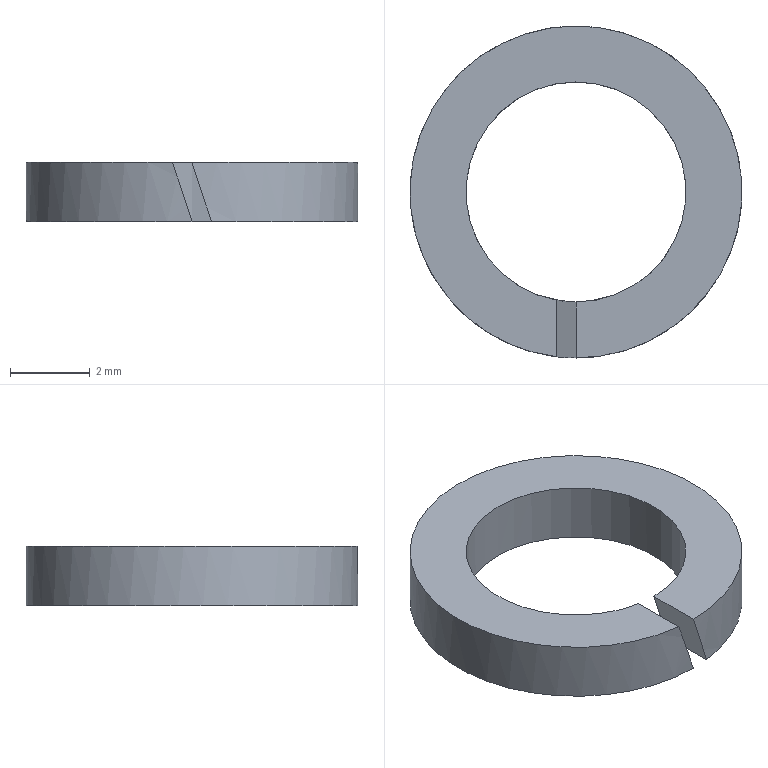Part | STEP file | 1_37 | 1 solid | 6 faces | box 8.3 x 8.3 x 1.5 mm | volume 44.494 mm3 | plane 4 | cylinder 2 | commonest cylinder face diameters 5.5 x1 8.3 x1
STEP:
#1=CARTESIAN_POINT('',(0.,0.,0.));
#2=DIRECTION('',(0.,0.,1.));
#3=DIRECTION('',(1.,0.,0.));
#4=AXIS2_PLACEMENT_3D('',#1,#2,#3);
#5=CARTESIAN_POINT('',(0.4882,-2.706,0.));
#6=VERTEX_POINT('',#5);
#7=CARTESIAN_POINT('',(0.,-2.75,1.5));
#8=VERTEX_POINT('',#7);
#9=CARTESIAN_POINT('',(-0.001613,0.01859,1.507));
#10=DIRECTION('',(-0.9509,0.0001849,-0.3095));
#11=DIRECTION('',(0.3095,-0.0002611,-0.9509));
#12=AXIS2_PLACEMENT_3D('',#9,#10,#11);
#13=ELLIPSE('',#12,8.915,2.769);
#14=CARTESIAN_POINT('',(0.,0.,0.75));
#15=DIRECTION('',(0.,0.,-1.));
#16=DIRECTION('',(1.,0.,0.));
#17=AXIS2_PLACEMENT_3D('',#14,#15,#16);
#18=CYLINDRICAL_SURFACE('',#17,2.75);
#19=CARTESIAN_POINT('',(7.675,0.75));
#20=CARTESIAN_POINT('',(7.854,-0.75));
#21=B_SPLINE_CURVE_WITH_KNOTS('',1,(#19,#20),.UNSPECIFIED.,.F.,.F.,(2,2),(1.392,1.57),.PIECEWISE_BEZIER_KNOTS.);
#22=(GEOMETRIC_REPRESENTATION_CONTEXT(2)PARAMETRIC_REPRESENTATION_CONTEXT()REPRESENTATION_CONTEXT('',''));
#23=DEFINITIONAL_REPRESENTATION('',(#21),#22);
#24=PCURVE('',#18,#23);
#25=CARTESIAN_POINT('',(0.,-2.61,1.5));
#26=DIRECTION('',(0.9509,0.,0.3095));
#27=DIRECTION('',(0.3095,0.,-0.9509));
#28=AXIS2_PLACEMENT_3D('',#25,#26,#27);
#29=PLANE('',#28);
#30=CARTESIAN_POINT('',(1.577,-0.09631));
#31=CARTESIAN_POINT('',(1.382,-0.1072));
#32=CARTESIAN_POINT('',(1.186,-0.1166));
#33=CARTESIAN_POINT('',(0.9897,-0.1244));
#34=CARTESIAN_POINT('',(0.7923,-0.1306));
#35=CARTESIAN_POINT('',(0.5946,-0.1353));
#36=CARTESIAN_POINT('',(0.3965,-0.1384));
#37=CARTESIAN_POINT('',(0.1982,-0.14));
#38=CARTESIAN_POINT('',(0.,-0.14));
#39=B_SPLINE_CURVE_WITH_KNOTS('',8,(#30,#31,#32,#33,#34,#35,#36,#37,#38),.UNSPECIFIED.,.F.,.F.,(9,9),(1.392,1.57),.PIECEWISE_BEZIER_KNOTS.);
#40=(GEOMETRIC_REPRESENTATION_CONTEXT(2)PARAMETRIC_REPRESENTATION_CONTEXT()REPRESENTATION_CONTEXT('',''));
#41=DEFINITIONAL_REPRESENTATION('',(#39),#40);
#42=PCURVE('',#29,#41);
#43=SURFACE_CURVE('',#13,(#24,#42),.PCURVE_S1.);
#44=EDGE_CURVE('',#6,#8,#43,.T.);
#45=ORIENTED_EDGE('',*,*,#44,.F.);
#46=CARTESIAN_POINT('',(0.,-2.75,0.));
#47=VERTEX_POINT('',#46);
#48=CARTESIAN_POINT('',(0.,0.,0.));
#49=DIRECTION('',(0.,0.,1.));
#50=DIRECTION('',(1.,0.,0.));
#51=AXIS2_PLACEMENT_3D('',#48,#49,#50);
#52=CIRCLE('',#51,2.75);
#53=CARTESIAN_POINT('',(12.566,0.75));
#54=DIRECTION('',(-1.,0.));
#55=VECTOR('',#54,1.);
#56=LINE('',#53,#55);
#57=(GEOMETRIC_REPRESENTATION_CONTEXT(2)PARAMETRIC_REPRESENTATION_CONTEXT()REPRESENTATION_CONTEXT('',''));
#58=DEFINITIONAL_REPRESENTATION('',(#56),#57);
#59=PCURVE('',#18,#58);
#60=CARTESIAN_POINT('',(3.45,0.,0.));
#61=DIRECTION('',(0.,0.,-1.));
#62=DIRECTION('',(-1.,0.,0.));
#63=AXIS2_PLACEMENT_3D('',#60,#61,#62);
#64=PLANE('',#63);
#65=CARTESIAN_POINT('',(0.7,0.));
#66=CARTESIAN_POINT('',(0.7,4.763));
#67=CARTESIAN_POINT('',(4.825,2.382));
#68=CARTESIAN_POINT('',(8.95,0.));
#69=CARTESIAN_POINT('',(4.825,-2.382));
#70=CARTESIAN_POINT('',(0.7,-4.763));
#71=CARTESIAN_POINT('',(0.7,0.));
#72=(BOUNDED_CURVE()B_SPLINE_CURVE(2,(#65,#66,#67,#68,#69,#70,#71),.UNSPECIFIED.,.T.,.F.)B_SPLINE_CURVE_WITH_KNOTS((1,2,2,2,2,1),(-2.094,0.,2.094,4.189,6.283,8.378),.UNSPECIFIED.)CURVE()GEOMETRIC_REPRESENTATION_ITEM()RATIONAL_B_SPLINE_CURVE((1.,0.5,1.,0.5,1.,0.5,1.))REPRESENTATION_ITEM(''));
#73=(GEOMETRIC_REPRESENTATION_CONTEXT(2)PARAMETRIC_REPRESENTATION_CONTEXT()REPRESENTATION_CONTEXT('',''));
#74=DEFINITIONAL_REPRESENTATION('',(#72),#73);
#75=PCURVE('',#64,#74);
#76=SURFACE_CURVE('',#52,(#59,#75),.PCURVE_S1.);
#77=EDGE_CURVE('',#6,#47,#76,.T.);
#78=ORIENTED_EDGE('',*,*,#77,.T.);
#79=CARTESIAN_POINT('',(-0.4882,-2.706,1.5));
#80=VERTEX_POINT('',#79);
#81=CARTESIAN_POINT('',(0.001613,0.01859,-0.006609));
#82=DIRECTION('',(0.9509,0.0001849,0.3095));
#83=DIRECTION('',(0.3095,0.0002611,-0.9509));
#84=AXIS2_PLACEMENT_3D('',#81,#82,#83);
#85=ELLIPSE('',#84,8.915,2.769);
#86=CARTESIAN_POINT('',(1.749,-0.75));
#87=CARTESIAN_POINT('',(1.571,0.75));
#88=B_SPLINE_CURVE_WITH_KNOTS('',1,(#86,#87),.UNSPECIFIED.,.F.,.F.,(2,2),(4.534,4.712),.PIECEWISE_BEZIER_KNOTS.);
#89=(GEOMETRIC_REPRESENTATION_CONTEXT(2)PARAMETRIC_REPRESENTATION_CONTEXT()REPRESENTATION_CONTEXT('',''));
#90=DEFINITIONAL_REPRESENTATION('',(#88),#89);
#91=PCURVE('',#18,#90);
#92=CARTESIAN_POINT('',(0.,-2.61,0.));
#93=DIRECTION('',(-0.9509,0.,-0.3095));
#94=DIRECTION('',(-0.3095,0.,0.9509));
#95=AXIS2_PLACEMENT_3D('',#92,#93,#94);
#96=PLANE('',#95);
#97=CARTESIAN_POINT('',(1.577,-0.09631));
#98=CARTESIAN_POINT('',(1.382,-0.1072));
#99=CARTESIAN_POINT('',(1.186,-0.1166));
#100=CARTESIAN_POINT('',(0.9897,-0.1244));
#101=CARTESIAN_POINT('',(0.7923,-0.1306));
#102=CARTESIAN_POINT('',(0.5946,-0.1353));
#103=CARTESIAN_POINT('',(0.3965,-0.1384));
#104=CARTESIAN_POINT('',(0.1982,-0.14));
#105=CARTESIAN_POINT('',(0.,-0.14));
#106=B_SPLINE_CURVE_WITH_KNOTS('',8,(#97,#98,#99,#100,#101,#102,#103,#104,#105),.UNSPECIFIED.,.F.,.F.,(9,9),(4.534,4.712),.PIECEWISE_BEZIER_KNOTS.);
#107=(GEOMETRIC_REPRESENTATION_CONTEXT(2)PARAMETRIC_REPRESENTATION_CONTEXT()REPRESENTATION_CONTEXT('',''));
#108=DEFINITIONAL_REPRESENTATION('',(#106),#107);
#109=PCURVE('',#96,#108);
#110=SURFACE_CURVE('',#85,(#91,#109),.PCURVE_S1.);
#111=EDGE_CURVE('',#80,#47,#110,.T.);
#112=ORIENTED_EDGE('',*,*,#111,.F.);
#113=CARTESIAN_POINT('',(0.,0.,1.5));
#114=DIRECTION('',(0.,0.,-1.));
#115=DIRECTION('',(1.,0.,0.));
#116=AXIS2_PLACEMENT_3D('',#113,#114,#115);
#117=CIRCLE('',#116,2.75);
#118=CARTESIAN_POINT('',(0.,-0.75));
#119=DIRECTION('',(1.,0.));
#120=VECTOR('',#119,1.);
#121=LINE('',#118,#120);
#122=(GEOMETRIC_REPRESENTATION_CONTEXT(2)PARAMETRIC_REPRESENTATION_CONTEXT()REPRESENTATION_CONTEXT('',''));
#123=DEFINITIONAL_REPRESENTATION('',(#121),#122);
#124=PCURVE('',#18,#123);
#125=CARTESIAN_POINT('',(3.45,0.,1.5));
#126=DIRECTION('',(0.,0.,1.));
#127=DIRECTION('',(1.,0.,0.));
#128=AXIS2_PLACEMENT_3D('',#125,#126,#127);
#129=PLANE('',#128);
#130=CARTESIAN_POINT('',(-0.7,0.));
#131=CARTESIAN_POINT('',(-0.7,-4.763));
#132=CARTESIAN_POINT('',(-4.825,-2.382));
#133=CARTESIAN_POINT('',(-8.95,0.));
#134=CARTESIAN_POINT('',(-4.825,2.382));
#135=CARTESIAN_POINT('',(-0.7,4.763));
#136=CARTESIAN_POINT('',(-0.7,0.));
#137=(BOUNDED_CURVE()B_SPLINE_CURVE(2,(#130,#131,#132,#133,#134,#135,#136),.UNSPECIFIED.,.T.,.F.)B_SPLINE_CURVE_WITH_KNOTS((1,2,2,2,2,1),(-2.094,0.,2.094,4.189,6.283,8.378),.UNSPECIFIED.)CURVE()GEOMETRIC_REPRESENTATION_ITEM()RATIONAL_B_SPLINE_CURVE((1.,0.5,1.,0.5,1.,0.5,1.))REPRESENTATION_ITEM(''));
#138=(GEOMETRIC_REPRESENTATION_CONTEXT(2)PARAMETRIC_REPRESENTATION_CONTEXT()REPRESENTATION_CONTEXT('',''));
#139=DEFINITIONAL_REPRESENTATION('',(#137),#138);
#140=PCURVE('',#129,#139);
#141=SURFACE_CURVE('',#117,(#124,#140),.PCURVE_S1.);
#142=EDGE_CURVE('',#80,#8,#141,.T.);
#143=ORIENTED_EDGE('',*,*,#142,.T.);
#144=EDGE_LOOP('',(#45,#78,#112,#143));
#145=FACE_BOUND('',#144,.F.);
#146=ADVANCED_FACE('',(#145),#18,.F.);
#147=CARTESIAN_POINT('',(0.,-4.15,1.5));
#148=VERTEX_POINT('',#147);
#149=CARTESIAN_POINT('',(0.000000001,-2.75,1.5));
#150=DIRECTION('',(0.,-1.,0.));
#151=VECTOR('',#150,1.);
#152=LINE('',#149,#151);
#153=CARTESIAN_POINT('',(-3.45,-2.75));
#154=DIRECTION('',(0.,-1.));
#155=VECTOR('',#154,1.);
#156=LINE('',#153,#155);
#157=(GEOMETRIC_REPRESENTATION_CONTEXT(2)PARAMETRIC_REPRESENTATION_CONTEXT()REPRESENTATION_CONTEXT('',''));
#158=DEFINITIONAL_REPRESENTATION('',(#156),#157);
#159=PCURVE('',#129,#158);
#160=CARTESIAN_POINT('',(0.,-0.14));
#161=DIRECTION('',(0.,-1.));
#162=VECTOR('',#161,1.);
#163=LINE('',#160,#162);
#164=(GEOMETRIC_REPRESENTATION_CONTEXT(2)PARAMETRIC_REPRESENTATION_CONTEXT()REPRESENTATION_CONTEXT('',''));
#165=DEFINITIONAL_REPRESENTATION('',(#163),#164);
#166=PCURVE('',#29,#165);
#167=SURFACE_CURVE('',#152,(#159,#166),.PCURVE_S1.);
#168=EDGE_CURVE('',#8,#148,#167,.T.);
#169=ORIENTED_EDGE('',*,*,#168,.T.);
#170=CARTESIAN_POINT('',(-0.4882,-4.121,1.5));
#171=VERTEX_POINT('',#170);
#172=CARTESIAN_POINT('',(-0.000000001,0.,1.5));
#173=DIRECTION('',(0.,0.,1.));
#174=DIRECTION('',(1.,0.,0.));
#175=AXIS2_PLACEMENT_3D('',#172,#173,#174);
#176=CIRCLE('',#175,4.15);
#177=CARTESIAN_POINT('',(-3.45,0.));
#178=DIRECTION('',(1.,0.));
#179=AXIS2_PLACEMENT_2D('',#177,#178);
#180=CIRCLE('',#179,4.15);
#181=(GEOMETRIC_REPRESENTATION_CONTEXT(2)PARAMETRIC_REPRESENTATION_CONTEXT()REPRESENTATION_CONTEXT('',''));
#182=DEFINITIONAL_REPRESENTATION('',(#180),#181);
#183=PCURVE('',#129,#182);
#184=CARTESIAN_POINT('',(0.,0.,0.75));
#185=DIRECTION('',(0.,0.,-1.));
#186=DIRECTION('',(1.,0.,0.));
#187=AXIS2_PLACEMENT_3D('',#184,#185,#186);
#188=CYLINDRICAL_SURFACE('',#187,4.15);
#189=CARTESIAN_POINT('',(12.566,-0.75));
#190=DIRECTION('',(-1.,0.));
#191=VECTOR('',#190,1.);
#192=LINE('',#189,#191);
#193=(GEOMETRIC_REPRESENTATION_CONTEXT(2)PARAMETRIC_REPRESENTATION_CONTEXT()REPRESENTATION_CONTEXT('',''));
#194=DEFINITIONAL_REPRESENTATION('',(#192),#193);
#195=PCURVE('',#188,#194);
#196=SURFACE_CURVE('',#176,(#183,#195),.PCURVE_S1.);
#197=EDGE_CURVE('',#148,#171,#196,.T.);
#198=ORIENTED_EDGE('',*,*,#197,.T.);
#199=CARTESIAN_POINT('',(-0.4882,-4.121,1.5));
#200=DIRECTION('',(0.,1.,0.));
#201=VECTOR('',#200,1.);
#202=LINE('',#199,#201);
#203=CARTESIAN_POINT('',(-3.938,-4.121));
#204=DIRECTION('',(0.,1.));
#205=VECTOR('',#204,1.);
#206=LINE('',#203,#205);
#207=(GEOMETRIC_REPRESENTATION_CONTEXT(2)PARAMETRIC_REPRESENTATION_CONTEXT()REPRESENTATION_CONTEXT('',''));
#208=DEFINITIONAL_REPRESENTATION('',(#206),#207);
#209=PCURVE('',#129,#208);
#210=CARTESIAN_POINT('',(1.577,-1.511));
#211=DIRECTION('',(0.,1.));
#212=VECTOR('',#211,1.);
#213=LINE('',#210,#212);
#214=(GEOMETRIC_REPRESENTATION_CONTEXT(2)PARAMETRIC_REPRESENTATION_CONTEXT()REPRESENTATION_CONTEXT('',''));
#215=DEFINITIONAL_REPRESENTATION('',(#213),#214);
#216=PCURVE('',#96,#215);
#217=SURFACE_CURVE('',#202,(#209,#216),.PCURVE_S1.);
#218=EDGE_CURVE('',#171,#80,#217,.T.);
#219=ORIENTED_EDGE('',*,*,#218,.T.);
#220=ORIENTED_EDGE('',*,*,#142,.T.);
#221=EDGE_LOOP('',(#169,#198,#219,#220));
#222=FACE_BOUND('',#221,.T.);
#223=ADVANCED_FACE('',(#222),#129,.T.);
#224=ORIENTED_EDGE('',*,*,#111,.F.);
#225=ORIENTED_EDGE('',*,*,#218,.F.);
#226=CARTESIAN_POINT('',(0.,-4.15,0.));
#227=VERTEX_POINT('',#226);
#228=CARTESIAN_POINT('',(-0.009565,-0.1621,0.02939));
#229=DIRECTION('',(-0.9509,0.,-0.3095));
#230=DIRECTION('',(0.3095,-0.0007855,-0.9509));
#231=AXIS2_PLACEMENT_3D('',#228,#229,#230);
#232=ELLIPSE('',#231,13.143,3.988);
#233=CARTESIAN_POINT('',(0.0309,2.448));
#234=DIRECTION('',(-1.,-0.0007855));
#235=AXIS2_PLACEMENT_2D('',#233,#234);
#236=ELLIPSE('',#235,13.143,3.988);
#237=(GEOMETRIC_REPRESENTATION_CONTEXT(2)PARAMETRIC_REPRESENTATION_CONTEXT()REPRESENTATION_CONTEXT('',''));
#238=DEFINITIONAL_REPRESENTATION('',(#236),#237);
#239=PCURVE('',#96,#238);
#240=CARTESIAN_POINT('',(1.571,0.75));
#241=CARTESIAN_POINT('',(1.689,-0.75));
#242=B_SPLINE_CURVE_WITH_KNOTS('',1,(#240,#241),.UNSPECIFIED.,.F.,.F.,(2,2),(1.568,1.689),.PIECEWISE_BEZIER_KNOTS.);
#243=(GEOMETRIC_REPRESENTATION_CONTEXT(2)PARAMETRIC_REPRESENTATION_CONTEXT()REPRESENTATION_CONTEXT('',''));
#244=DEFINITIONAL_REPRESENTATION('',(#242),#243);
#245=PCURVE('',#188,#244);
#246=SURFACE_CURVE('',#232,(#239,#245),.PCURVE_S1.);
#247=EDGE_CURVE('',#227,#171,#246,.T.);
#248=ORIENTED_EDGE('',*,*,#247,.F.);
#249=CARTESIAN_POINT('',(0.,-2.75,0.));
#250=DIRECTION('',(0.,-1.,0.));
#251=VECTOR('',#250,1.);
#252=LINE('',#249,#251);
#253=CARTESIAN_POINT('',(0.,-0.14));
#254=DIRECTION('',(0.,-1.));
#255=VECTOR('',#254,1.);
#256=LINE('',#253,#255);
#257=(GEOMETRIC_REPRESENTATION_CONTEXT(2)PARAMETRIC_REPRESENTATION_CONTEXT()REPRESENTATION_CONTEXT('',''));
#258=DEFINITIONAL_REPRESENTATION('',(#256),#257);
#259=PCURVE('',#96,#258);
#260=CARTESIAN_POINT('',(3.45,-2.75));
#261=DIRECTION('',(0.,-1.));
#262=VECTOR('',#261,1.);
#263=LINE('',#260,#262);
#264=(GEOMETRIC_REPRESENTATION_CONTEXT(2)PARAMETRIC_REPRESENTATION_CONTEXT()REPRESENTATION_CONTEXT('',''));
#265=DEFINITIONAL_REPRESENTATION('',(#263),#264);
#266=PCURVE('',#64,#265);
#267=SURFACE_CURVE('',#252,(#259,#266),.PCURVE_S1.);
#268=EDGE_CURVE('',#47,#227,#267,.T.);
#269=ORIENTED_EDGE('',*,*,#268,.F.);
#270=EDGE_LOOP('',(#224,#225,#248,#269));
#271=FACE_BOUND('',#270,.T.);
#272=ADVANCED_FACE('',(#271),#96,.F.);
#273=CARTESIAN_POINT('',(0.4882,-4.121,0.000000001));
#274=VERTEX_POINT('',#273);
#275=CARTESIAN_POINT('',(0.4882,-4.121,0.));
#276=DIRECTION('',(0.,1.,0.));
#277=VECTOR('',#276,1.);
#278=LINE('',#275,#277);
#279=CARTESIAN_POINT('',(2.962,-4.121));
#280=DIRECTION('',(0.,1.));
#281=VECTOR('',#280,1.);
#282=LINE('',#279,#281);
#283=(GEOMETRIC_REPRESENTATION_CONTEXT(2)PARAMETRIC_REPRESENTATION_CONTEXT()REPRESENTATION_CONTEXT('',''));
#284=DEFINITIONAL_REPRESENTATION('',(#282),#283);
#285=PCURVE('',#64,#284);
#286=CARTESIAN_POINT('',(1.577,-1.511));
#287=DIRECTION('',(0.,1.));
#288=VECTOR('',#287,1.);
#289=LINE('',#286,#288);
#290=(GEOMETRIC_REPRESENTATION_CONTEXT(2)PARAMETRIC_REPRESENTATION_CONTEXT()REPRESENTATION_CONTEXT('',''));
#291=DEFINITIONAL_REPRESENTATION('',(#289),#290);
#292=PCURVE('',#29,#291);
#293=SURFACE_CURVE('',#278,(#285,#292),.PCURVE_S1.);
#294=EDGE_CURVE('',#274,#6,#293,.T.);
#295=ORIENTED_EDGE('',*,*,#294,.T.);
#296=ORIENTED_EDGE('',*,*,#77,.T.);
#297=ORIENTED_EDGE('',*,*,#268,.T.);
#298=CARTESIAN_POINT('',(0.,0.,0.));
#299=DIRECTION('',(0.,0.,1.));
#300=DIRECTION('',(0.,-1.,0.));
#301=AXIS2_PLACEMENT_3D('',#298,#299,#300);
#302=CIRCLE('',#301,4.15);
#303=CARTESIAN_POINT('',(3.45,-4.15));
#304=CARTESIAN_POINT('',(-3.738,-4.15));
#305=CARTESIAN_POINT('',(-0.144,2.075));
#306=CARTESIAN_POINT('',(3.45,8.3));
#307=CARTESIAN_POINT('',(7.044,2.075));
#308=CARTESIAN_POINT('',(10.638,-4.15));
#309=CARTESIAN_POINT('',(3.45,-4.15));
#310=(BOUNDED_CURVE()B_SPLINE_CURVE(2,(#303,#304,#305,#306,#307,#308,#309),.UNSPECIFIED.,.T.,.F.)B_SPLINE_CURVE_WITH_KNOTS((1,2,2,2,2,1),(-2.094,0.,2.094,4.189,6.283,8.378),.UNSPECIFIED.)CURVE()GEOMETRIC_REPRESENTATION_ITEM()RATIONAL_B_SPLINE_CURVE((1.,0.5,1.,0.5,1.,0.5,1.))REPRESENTATION_ITEM(''));
#311=(GEOMETRIC_REPRESENTATION_CONTEXT(2)PARAMETRIC_REPRESENTATION_CONTEXT()REPRESENTATION_CONTEXT('',''));
#312=DEFINITIONAL_REPRESENTATION('',(#310),#311);
#313=PCURVE('',#64,#312);
#314=CARTESIAN_POINT('',(7.854,0.75));
#315=DIRECTION('',(-1.,0.));
#316=VECTOR('',#315,1.);
#317=LINE('',#314,#316);
#318=(GEOMETRIC_REPRESENTATION_CONTEXT(2)PARAMETRIC_REPRESENTATION_CONTEXT()REPRESENTATION_CONTEXT('',''));
#319=DEFINITIONAL_REPRESENTATION('',(#317),#318);
#320=PCURVE('',#188,#319);
#321=SURFACE_CURVE('',#302,(#313,#320),.PCURVE_S1.);
#322=EDGE_CURVE('',#274,#227,#321,.T.);
#323=ORIENTED_EDGE('',*,*,#322,.F.);
#324=EDGE_LOOP('',(#295,#296,#297,#323));
#325=FACE_BOUND('',#324,.T.);
#326=ADVANCED_FACE('',(#325),#64,.T.);
#327=ORIENTED_EDGE('',*,*,#44,.F.);
#328=ORIENTED_EDGE('',*,*,#294,.F.);
#329=CARTESIAN_POINT('',(0.009565,-0.1621,1.471));
#330=DIRECTION('',(0.9509,0.,0.3095));
#331=DIRECTION('',(0.3095,0.0007855,-0.9509));
#332=AXIS2_PLACEMENT_3D('',#329,#330,#331);
#333=ELLIPSE('',#332,13.143,3.988);
#334=CARTESIAN_POINT('',(0.0309,2.448));
#335=DIRECTION('',(1.,0.0007855));
#336=AXIS2_PLACEMENT_2D('',#334,#335);
#337=ELLIPSE('',#336,13.143,3.988);
#338=(GEOMETRIC_REPRESENTATION_CONTEXT(2)PARAMETRIC_REPRESENTATION_CONTEXT()REPRESENTATION_CONTEXT('',''));
#339=DEFINITIONAL_REPRESENTATION('',(#337),#338);
#340=PCURVE('',#29,#339);
#341=CARTESIAN_POINT('',(7.854,-0.75));
#342=CARTESIAN_POINT('',(7.736,0.75));
#343=B_SPLINE_CURVE_WITH_KNOTS('',1,(#341,#342),.UNSPECIFIED.,.F.,.F.,(2,2),(4.71,4.83),.PIECEWISE_BEZIER_KNOTS.);
#344=(GEOMETRIC_REPRESENTATION_CONTEXT(2)PARAMETRIC_REPRESENTATION_CONTEXT()REPRESENTATION_CONTEXT('',''));
#345=DEFINITIONAL_REPRESENTATION('',(#343),#344);
#346=PCURVE('',#188,#345);
#347=SURFACE_CURVE('',#333,(#340,#346),.PCURVE_S1.);
#348=EDGE_CURVE('',#148,#274,#347,.T.);
#349=ORIENTED_EDGE('',*,*,#348,.F.);
#350=ORIENTED_EDGE('',*,*,#168,.F.);
#351=EDGE_LOOP('',(#327,#328,#349,#350));
#352=FACE_BOUND('',#351,.T.);
#353=ADVANCED_FACE('',(#352),#29,.F.);
#354=ORIENTED_EDGE('',*,*,#197,.F.);
#355=ORIENTED_EDGE('',*,*,#348,.T.);
#356=ORIENTED_EDGE('',*,*,#322,.T.);
#357=ORIENTED_EDGE('',*,*,#247,.T.);
#358=EDGE_LOOP('',(#354,#355,#356,#357));
#359=FACE_BOUND('',#358,.T.);
#360=ADVANCED_FACE('',(#359),#188,.T.);
#361=CLOSED_SHELL('',(#146,#223,#272,#326,#353,#360));
#362=MANIFOLD_SOLID_BREP('',#361);
#363=(LENGTH_UNIT()NAMED_UNIT(*)SI_UNIT(.MILLI.,.METRE.));
#364=UNCERTAINTY_MEASURE_WITH_UNIT(LENGTH_MEASURE(0.002),#363,'','');
#365=(NAMED_UNIT(*)PLANE_ANGLE_UNIT()SI_UNIT($,.RADIAN.));
#366=(NAMED_UNIT(*)SI_UNIT($,.STERADIAN.)SOLID_ANGLE_UNIT());
#367=(GEOMETRIC_REPRESENTATION_CONTEXT(3)GLOBAL_UNCERTAINTY_ASSIGNED_CONTEXT((#364))GLOBAL_UNIT_ASSIGNED_CONTEXT((#363,#365,#366))REPRESENTATION_CONTEXT('',''));
#368=ADVANCED_BREP_SHAPE_REPRESENTATION('',(#4,#362),#367);